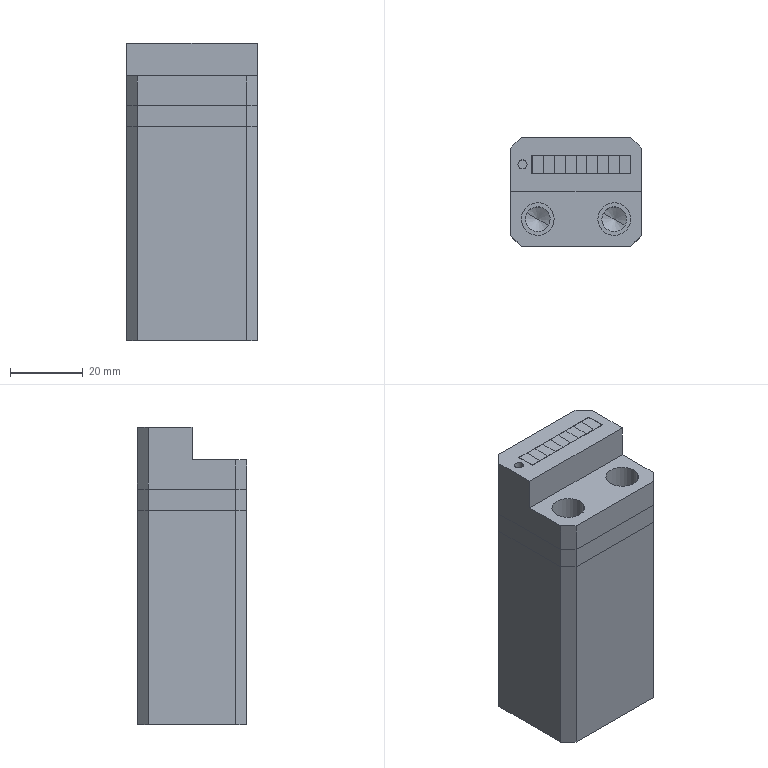Part | CATIA | 12 solids | 164 faces | box 36 x 30 x 81.8 mm | volume 74943 mm3 | plane 130 | cylinder 24 | cone 10 | commonest cylinder face diameters 6.8 x10 9 x8 2.5 x4 6 x2